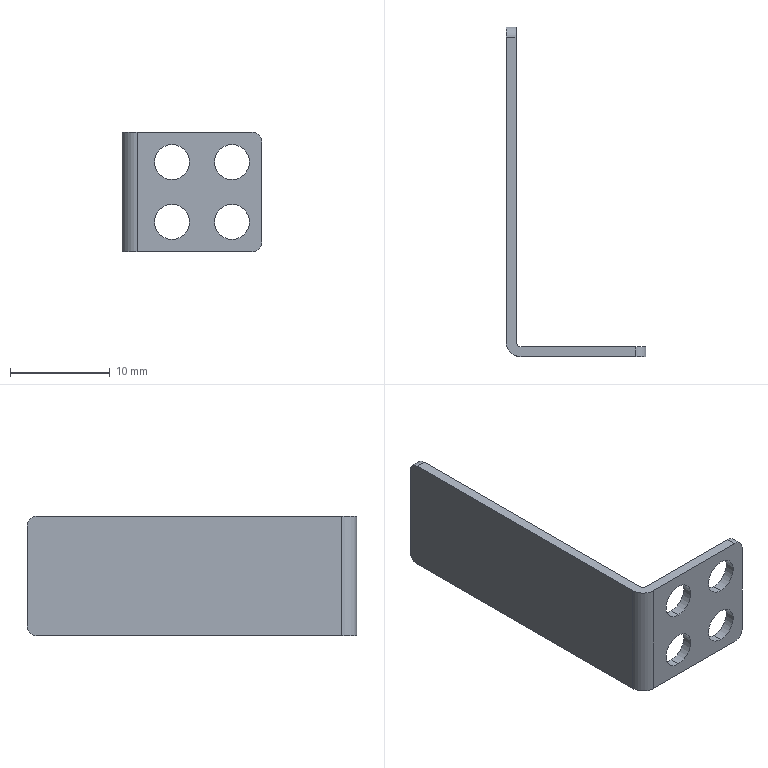Part | SolidWorks | features MoveFace 7, ICE 2, BaseBody 1, Fillet 1 | 1 solid | 22 faces | box 14 x 33 x 12 mm | volume 507.507 mm3 | cylinder 14 | plane 8 | commonest cylinder face diameters 3.5 x8 2 x4 1 x1 3 x1
STEP:
#1=CARTESIAN_POINT('',(4.,-12.5,-9.25));
#2=VERTEX_POINT('',#1);
#3=CARTESIAN_POINT('',(4.,-12.5,-12.75));
#4=VERTEX_POINT('',#3);
#5=CARTESIAN_POINT('',(4.,-12.5,-11.));
#6=DIRECTION('',(0.,-1.,0.));
#7=DIRECTION('',(0.,0.,-1.));
#8=AXIS2_PLACEMENT_3D('',#5,#6,#7);
#9=CIRCLE('',#8,1.75);
#10=EDGE_CURVE('',#2,#4,#9,.T.);
#11=ORIENTED_EDGE('',*,*,#10,.T.);
#12=CARTESIAN_POINT('',(4.,-11.5,-12.75));
#13=VERTEX_POINT('',#12);
#14=CARTESIAN_POINT('',(4.,-21.5,-12.75));
#15=DIRECTION('',(0.,1.,0.));
#16=VECTOR('',#15,1000.);
#17=LINE('',#14,#16);
#18=EDGE_CURVE('',#4,#13,#17,.T.);
#19=ORIENTED_EDGE('',*,*,#18,.T.);
#20=CARTESIAN_POINT('',(4.,-11.5,-9.25));
#21=VERTEX_POINT('',#20);
#22=CARTESIAN_POINT('',(4.,-11.5,-11.));
#23=DIRECTION('',(0.,1.,0.));
#24=DIRECTION('',(0.,0.,1.));
#25=AXIS2_PLACEMENT_3D('',#22,#23,#24);
#26=CIRCLE('',#25,1.75);
#27=EDGE_CURVE('',#13,#21,#26,.T.);
#28=ORIENTED_EDGE('',*,*,#27,.T.);
#29=CARTESIAN_POINT('',(4.,-21.5,-9.25));
#30=DIRECTION('',(0.,1.,0.));
#31=VECTOR('',#30,1000.);
#32=LINE('',#29,#31);
#33=EDGE_CURVE('',#2,#21,#32,.T.);
#34=ORIENTED_EDGE('',*,*,#33,.F.);
#35=EDGE_LOOP('',(#11,#19,#28,#34));
#36=FACE_OUTER_BOUND('',#35,.T.);
#37=CARTESIAN_POINT('',(4.,-21.5,-11.));
#38=DIRECTION('',(0.,1.,0.));
#39=DIRECTION('',(0.,0.,1.));
#40=AXIS2_PLACEMENT_3D('',#37,#38,#39);
#41=CYLINDRICAL_SURFACE('',#40,1.75);
#42=ADVANCED_FACE('',(#36),#41,.F.);
#43=CARTESIAN_POINT('',(-2.,-12.5,-12.75));
#44=VERTEX_POINT('',#43);
#45=CARTESIAN_POINT('',(-2.,-12.5,-9.25));
#46=VERTEX_POINT('',#45);
#47=CARTESIAN_POINT('',(-2.,-12.5,-11.));
#48=DIRECTION('',(0.,1.,0.));
#49=DIRECTION('',(0.,0.,1.));
#50=AXIS2_PLACEMENT_3D('',#47,#48,#49);
#51=CIRCLE('',#50,1.75);
#52=EDGE_CURVE('',#44,#46,#51,.T.);
#53=ORIENTED_EDGE('',*,*,#52,.F.);
#54=CARTESIAN_POINT('',(-2.,-11.5,-12.75));
#55=VERTEX_POINT('',#54);
#56=CARTESIAN_POINT('',(-2.,-11.5,-12.75));
#57=DIRECTION('',(0.,1.,0.));
#58=VECTOR('',#57,1000.);
#59=LINE('',#56,#58);
#60=EDGE_CURVE('',#44,#55,#59,.T.);
#61=ORIENTED_EDGE('',*,*,#60,.T.);
#62=CARTESIAN_POINT('',(-2.,-11.5,-9.25));
#63=VERTEX_POINT('',#62);
#64=CARTESIAN_POINT('',(-2.,-11.5,-11.));
#65=DIRECTION('',(0.,1.,0.));
#66=DIRECTION('',(0.,0.,1.));
#67=AXIS2_PLACEMENT_3D('',#64,#65,#66);
#68=CIRCLE('',#67,1.75);
#69=EDGE_CURVE('',#55,#63,#68,.T.);
#70=ORIENTED_EDGE('',*,*,#69,.T.);
#71=CARTESIAN_POINT('',(-2.,-11.5,-9.25));
#72=DIRECTION('',(0.,1.,0.));
#73=VECTOR('',#72,1000.);
#74=LINE('',#71,#73);
#75=EDGE_CURVE('',#46,#63,#74,.T.);
#76=ORIENTED_EDGE('',*,*,#75,.F.);
#77=EDGE_LOOP('',(#53,#61,#70,#76));
#78=FACE_OUTER_BOUND('',#77,.T.);
#79=CARTESIAN_POINT('',(-2.,-11.5,-11.));
#80=DIRECTION('',(0.,1.,0.));
#81=DIRECTION('',(0.,0.,1.));
#82=AXIS2_PLACEMENT_3D('',#79,#80,#81);
#83=CYLINDRICAL_SURFACE('',#82,1.75);
#84=ADVANCED_FACE('',(#78),#83,.F.);
#85=CARTESIAN_POINT('',(4.,-12.5,-6.75));
#86=VERTEX_POINT('',#85);
#87=CARTESIAN_POINT('',(4.,-12.5,-3.25));
#88=VERTEX_POINT('',#87);
#89=CARTESIAN_POINT('',(4.,-12.5,-5.));
#90=DIRECTION('',(0.,1.,0.));
#91=DIRECTION('',(0.,0.,1.));
#92=AXIS2_PLACEMENT_3D('',#89,#90,#91);
#93=CIRCLE('',#92,1.75);
#94=EDGE_CURVE('',#86,#88,#93,.T.);
#95=ORIENTED_EDGE('',*,*,#94,.F.);
#96=CARTESIAN_POINT('',(4.,-11.5,-6.75));
#97=VERTEX_POINT('',#96);
#98=CARTESIAN_POINT('',(4.,-11.5,-6.75));
#99=DIRECTION('',(0.,1.,0.));
#100=VECTOR('',#99,1000.);
#101=LINE('',#98,#100);
#102=EDGE_CURVE('',#86,#97,#101,.T.);
#103=ORIENTED_EDGE('',*,*,#102,.T.);
#104=CARTESIAN_POINT('',(4.,-11.5,-3.25));
#105=VERTEX_POINT('',#104);
#106=CARTESIAN_POINT('',(4.,-11.5,-5.));
#107=DIRECTION('',(0.,1.,0.));
#108=DIRECTION('',(0.,0.,1.));
#109=AXIS2_PLACEMENT_3D('',#106,#107,#108);
#110=CIRCLE('',#109,1.75);
#111=EDGE_CURVE('',#97,#105,#110,.T.);
#112=ORIENTED_EDGE('',*,*,#111,.T.);
#113=CARTESIAN_POINT('',(4.,-11.5,-3.25));
#114=DIRECTION('',(0.,1.,0.));
#115=VECTOR('',#114,1000.);
#116=LINE('',#113,#115);
#117=EDGE_CURVE('',#88,#105,#116,.T.);
#118=ORIENTED_EDGE('',*,*,#117,.F.);
#119=EDGE_LOOP('',(#95,#103,#112,#118));
#120=FACE_OUTER_BOUND('',#119,.T.);
#121=CARTESIAN_POINT('',(4.,-11.5,-5.));
#122=DIRECTION('',(0.,1.,0.));
#123=DIRECTION('',(0.,0.,1.));
#124=AXIS2_PLACEMENT_3D('',#121,#122,#123);
#125=CYLINDRICAL_SURFACE('',#124,1.75);
#126=ADVANCED_FACE('',(#120),#125,.F.);
#127=CARTESIAN_POINT('',(-2.,-12.5,-6.75));
#128=VERTEX_POINT('',#127);
#129=CARTESIAN_POINT('',(-2.,-12.5,-3.25));
#130=VERTEX_POINT('',#129);
#131=CARTESIAN_POINT('',(-2.,-12.5,-5.));
#132=DIRECTION('',(0.,1.,0.));
#133=DIRECTION('',(0.,0.,1.));
#134=AXIS2_PLACEMENT_3D('',#131,#132,#133);
#135=CIRCLE('',#134,1.75);
#136=EDGE_CURVE('',#128,#130,#135,.T.);
#137=ORIENTED_EDGE('',*,*,#136,.F.);
#138=CARTESIAN_POINT('',(-2.,-11.5,-6.75));
#139=VERTEX_POINT('',#138);
#140=CARTESIAN_POINT('',(-2.,-11.5,-6.75));
#141=DIRECTION('',(0.,1.,0.));
#142=VECTOR('',#141,1000.);
#143=LINE('',#140,#142);
#144=EDGE_CURVE('',#128,#139,#143,.T.);
#145=ORIENTED_EDGE('',*,*,#144,.T.);
#146=CARTESIAN_POINT('',(-2.,-11.5,-3.25));
#147=VERTEX_POINT('',#146);
#148=CARTESIAN_POINT('',(-2.,-11.5,-5.));
#149=DIRECTION('',(0.,1.,0.));
#150=DIRECTION('',(0.,0.,1.));
#151=AXIS2_PLACEMENT_3D('',#148,#149,#150);
#152=CIRCLE('',#151,1.75);
#153=EDGE_CURVE('',#139,#147,#152,.T.);
#154=ORIENTED_EDGE('',*,*,#153,.T.);
#155=CARTESIAN_POINT('',(-2.,-11.5,-3.25));
#156=DIRECTION('',(0.,1.,0.));
#157=VECTOR('',#156,1000.);
#158=LINE('',#155,#157);
#159=EDGE_CURVE('',#130,#147,#158,.T.);
#160=ORIENTED_EDGE('',*,*,#159,.F.);
#161=EDGE_LOOP('',(#137,#145,#154,#160));
#162=FACE_OUTER_BOUND('',#161,.T.);
#163=CARTESIAN_POINT('',(-2.,-11.5,-5.));
#164=DIRECTION('',(0.,1.,0.));
#165=DIRECTION('',(0.,0.,1.));
#166=AXIS2_PLACEMENT_3D('',#163,#164,#165);
#167=CYLINDRICAL_SURFACE('',#166,1.75);
#168=ADVANCED_FACE('',(#162),#167,.F.);
#169=CARTESIAN_POINT('',(-6.,20.5,-13.));
#170=VERTEX_POINT('',#169);
#171=CARTESIAN_POINT('',(-6.,19.5,-14.));
#172=VERTEX_POINT('',#171);
#173=CARTESIAN_POINT('',(-6.,19.5,-13.));
#174=DIRECTION('',(-1.,0.,0.));
#175=DIRECTION('',(0.,0.,-1.));
#176=AXIS2_PLACEMENT_3D('',#173,#174,#175);
#177=CIRCLE('',#176,1.);
#178=EDGE_CURVE('',#170,#172,#177,.T.);
#179=ORIENTED_EDGE('',*,*,#178,.F.);
#180=CARTESIAN_POINT('',(-6.,20.5,-3.));
#181=VERTEX_POINT('',#180);
#182=CARTESIAN_POINT('',(-6.,20.5,-15.));
#183=DIRECTION('',(0.,0.,-1.));
#184=VECTOR('',#183,1000.);
#185=LINE('',#182,#184);
#186=EDGE_CURVE('',#181,#170,#185,.T.);
#187=ORIENTED_EDGE('',*,*,#186,.F.);
#188=CARTESIAN_POINT('',(-6.,19.5,-2.));
#189=VERTEX_POINT('',#188);
#190=CARTESIAN_POINT('',(-6.,19.5,-3.));
#191=DIRECTION('',(-1.,0.,0.));
#192=DIRECTION('',(0.,0.,1.));
#193=AXIS2_PLACEMENT_3D('',#190,#191,#192);
#194=CIRCLE('',#193,1.);
#195=EDGE_CURVE('',#189,#181,#194,.T.);
#196=ORIENTED_EDGE('',*,*,#195,.F.);
#197=CARTESIAN_POINT('',(-6.,-11.,-2.));
#198=VERTEX_POINT('',#197);
#199=CARTESIAN_POINT('',(-6.,25.632,-2.));
#200=DIRECTION('',(0.,1.,0.));
#201=VECTOR('',#200,1000.);
#202=LINE('',#199,#201);
#203=EDGE_CURVE('',#198,#189,#202,.T.);
#204=ORIENTED_EDGE('',*,*,#203,.F.);
#205=CARTESIAN_POINT('',(-6.,-11.,-14.));
#206=VERTEX_POINT('',#205);
#207=CARTESIAN_POINT('',(-6.,-11.,-15.));
#208=DIRECTION('',(0.,0.,1.));
#209=VECTOR('',#208,1000.);
#210=LINE('',#207,#209);
#211=EDGE_CURVE('',#206,#198,#210,.T.);
#212=ORIENTED_EDGE('',*,*,#211,.F.);
#213=CARTESIAN_POINT('',(-6.,25.632,-14.));
#214=DIRECTION('',(0.,-1.,0.));
#215=VECTOR('',#214,1000.);
#216=LINE('',#213,#215);
#217=EDGE_CURVE('',#172,#206,#216,.T.);
#218=ORIENTED_EDGE('',*,*,#217,.F.);
#219=EDGE_LOOP('',(#179,#187,#196,#204,#212,#218));
#220=FACE_OUTER_BOUND('',#219,.T.);
#221=CARTESIAN_POINT('',(-6.,25.632,-15.));
#222=DIRECTION('',(-1.,0.,0.));
#223=DIRECTION('',(0.,-1.,0.));
#224=AXIS2_PLACEMENT_3D('',#221,#222,#223);
#225=PLANE('',#224);
#226=ADVANCED_FACE('',(#220),#225,.F.);
#227=CARTESIAN_POINT('',(-5.5,-11.5,-14.));
#228=VERTEX_POINT('',#227);
#229=CARTESIAN_POINT('',(6.,-11.5,-14.));
#230=VERTEX_POINT('',#229);
#231=CARTESIAN_POINT('',(28.84,-11.5,-14.));
#232=DIRECTION('',(1.,0.,0.));
#233=VECTOR('',#232,1000.);
#234=LINE('',#231,#233);
#235=EDGE_CURVE('',#228,#230,#234,.T.);
#236=ORIENTED_EDGE('',*,*,#235,.T.);
#237=CARTESIAN_POINT('',(6.,-12.5,-14.));
#238=VERTEX_POINT('',#237);
#239=CARTESIAN_POINT('',(6.,-12.5,-14.));
#240=DIRECTION('',(0.,-1.,0.));
#241=VECTOR('',#240,1000.);
#242=LINE('',#239,#241);
#243=EDGE_CURVE('',#230,#238,#242,.T.);
#244=ORIENTED_EDGE('',*,*,#243,.T.);
#245=CARTESIAN_POINT('',(-5.5,-12.5,-14.));
#246=VERTEX_POINT('',#245);
#247=CARTESIAN_POINT('',(-7.,-12.5,-14.));
#248=DIRECTION('',(1.,0.,0.));
#249=VECTOR('',#248,1000.);
#250=LINE('',#247,#249);
#251=EDGE_CURVE('',#246,#238,#250,.T.);
#252=ORIENTED_EDGE('',*,*,#251,.F.);
#253=CARTESIAN_POINT('',(-7.,-11.,-14.));
#254=VERTEX_POINT('',#253);
#255=CARTESIAN_POINT('',(-5.5,-11.,-14.));
#256=DIRECTION('',(0.,0.,1.));
#257=DIRECTION('',(1.,0.,0.));
#258=AXIS2_PLACEMENT_3D('',#255,#256,#257);
#259=CIRCLE('',#258,1.5);
#260=EDGE_CURVE('',#254,#246,#259,.T.);
#261=ORIENTED_EDGE('',*,*,#260,.F.);
#262=CARTESIAN_POINT('',(-7.,19.5,-14.));
#263=VERTEX_POINT('',#262);
#264=CARTESIAN_POINT('',(-7.,12.5,-14.));
#265=DIRECTION('',(0.,-1.,0.));
#266=VECTOR('',#265,1000.);
#267=LINE('',#264,#266);
#268=EDGE_CURVE('',#263,#254,#267,.T.);
#269=ORIENTED_EDGE('',*,*,#268,.F.);
#270=CARTESIAN_POINT('',(-5.,19.5,-14.));
#271=DIRECTION('',(-1.,0.,0.));
#272=VECTOR('',#271,1000.);
#273=LINE('',#270,#272);
#274=EDGE_CURVE('',#172,#263,#273,.T.);
#275=ORIENTED_EDGE('',*,*,#274,.F.);
#276=ORIENTED_EDGE('',*,*,#217,.T.);
#277=CARTESIAN_POINT('',(-5.5,-11.,-14.));
#278=DIRECTION('',(0.,0.,-1.));
#279=DIRECTION('',(-1.,0.,0.));
#280=AXIS2_PLACEMENT_3D('',#277,#278,#279);
#281=CIRCLE('',#280,0.5);
#282=EDGE_CURVE('',#228,#206,#281,.T.);
#283=ORIENTED_EDGE('',*,*,#282,.F.);
#284=EDGE_LOOP('',(#236,#244,#252,#261,#269,#275,#276,#283));
#285=FACE_OUTER_BOUND('',#284,.T.);
#286=CARTESIAN_POINT('',(-5.,12.5,-14.));
#287=DIRECTION('',(0.,0.,1.));
#288=DIRECTION('',(1.,0.,0.));
#289=AXIS2_PLACEMENT_3D('',#286,#287,#288);
#290=PLANE('',#289);
#291=ADVANCED_FACE('',(#285),#290,.F.);
#292=CARTESIAN_POINT('',(-7.,20.5,-13.));
#293=VERTEX_POINT('',#292);
#294=CARTESIAN_POINT('',(-7.,19.5,-13.));
#295=DIRECTION('',(1.,0.,0.));
#296=DIRECTION('',(0.,0.,-1.));
#297=AXIS2_PLACEMENT_3D('',#294,#295,#296);
#298=CIRCLE('',#297,1.);
#299=EDGE_CURVE('',#263,#293,#298,.T.);
#300=ORIENTED_EDGE('',*,*,#299,.T.);
#301=CARTESIAN_POINT('',(-7.,20.5,-13.));
#302=DIRECTION('',(1.,0.,0.));
#303=VECTOR('',#302,1000.);
#304=LINE('',#301,#303);
#305=EDGE_CURVE('',#293,#170,#304,.T.);
#306=ORIENTED_EDGE('',*,*,#305,.T.);
#307=ORIENTED_EDGE('',*,*,#178,.T.);
#308=ORIENTED_EDGE('',*,*,#274,.T.);
#309=EDGE_LOOP('',(#300,#306,#307,#308));
#310=FACE_OUTER_BOUND('',#309,.T.);
#311=CARTESIAN_POINT('',(-7.,19.5,-13.));
#312=DIRECTION('',(1.,0.,0.));
#313=DIRECTION('',(0.,0.,-1.));
#314=AXIS2_PLACEMENT_3D('',#311,#312,#313);
#315=CYLINDRICAL_SURFACE('',#314,1.);
#316=ADVANCED_FACE('',(#310),#315,.T.);
#317=CARTESIAN_POINT('',(-7.,20.5,-3.));
#318=VERTEX_POINT('',#317);
#319=CARTESIAN_POINT('',(-7.,20.5,-15.));
#320=DIRECTION('',(0.,0.,1.));
#321=VECTOR('',#320,1000.);
#322=LINE('',#319,#321);
#323=EDGE_CURVE('',#293,#318,#322,.T.);
#324=ORIENTED_EDGE('',*,*,#323,.T.);
#325=CARTESIAN_POINT('',(-7.,20.5,-3.));
#326=DIRECTION('',(1.,0.,0.));
#327=VECTOR('',#326,1000.);
#328=LINE('',#325,#327);
#329=EDGE_CURVE('',#318,#181,#328,.T.);
#330=ORIENTED_EDGE('',*,*,#329,.T.);
#331=ORIENTED_EDGE('',*,*,#186,.T.);
#332=ORIENTED_EDGE('',*,*,#305,.F.);
#333=EDGE_LOOP('',(#324,#330,#331,#332));
#334=FACE_OUTER_BOUND('',#333,.T.);
#335=CARTESIAN_POINT('',(-7.,20.5,-15.));
#336=DIRECTION('',(0.,1.,0.));
#337=DIRECTION('',(0.,0.,1.));
#338=AXIS2_PLACEMENT_3D('',#335,#336,#337);
#339=PLANE('',#338);
#340=ADVANCED_FACE('',(#334),#339,.T.);
#341=CARTESIAN_POINT('',(-7.,19.5,-2.));
#342=VERTEX_POINT('',#341);
#343=CARTESIAN_POINT('',(-7.,19.5,-3.));
#344=DIRECTION('',(1.,0.,0.));
#345=DIRECTION('',(0.,0.,1.));
#346=AXIS2_PLACEMENT_3D('',#343,#344,#345);
#347=CIRCLE('',#346,1.);
#348=EDGE_CURVE('',#318,#342,#347,.T.);
#349=ORIENTED_EDGE('',*,*,#348,.T.);
#350=CARTESIAN_POINT('',(0.,19.5,-2.));
#351=DIRECTION('',(1.,0.,0.));
#352=VECTOR('',#351,1000.);
#353=LINE('',#350,#352);
#354=EDGE_CURVE('',#342,#189,#353,.T.);
#355=ORIENTED_EDGE('',*,*,#354,.T.);
#356=ORIENTED_EDGE('',*,*,#195,.T.);
#357=ORIENTED_EDGE('',*,*,#329,.F.);
#358=EDGE_LOOP('',(#349,#355,#356,#357));
#359=FACE_OUTER_BOUND('',#358,.T.);
#360=CARTESIAN_POINT('',(0.,19.5,-3.));
#361=DIRECTION('',(-1.,0.,0.));
#362=DIRECTION('',(0.,0.,1.));
#363=AXIS2_PLACEMENT_3D('',#360,#361,#362);
#364=CYLINDRICAL_SURFACE('',#363,1.);
#365=ADVANCED_FACE('',(#359),#364,.T.);
#366=CARTESIAN_POINT('',(6.,-11.5,-2.));
#367=VERTEX_POINT('',#366);
#368=CARTESIAN_POINT('',(-5.5,-11.5,-2.));
#369=VERTEX_POINT('',#368);
#370=CARTESIAN_POINT('',(0.,-11.5,-2.));
#371=DIRECTION('',(-1.,0.,0.));
#372=VECTOR('',#371,1000.);
#373=LINE('',#370,#372);
#374=EDGE_CURVE('',#367,#369,#373,.T.);
#375=ORIENTED_EDGE('',*,*,#374,.T.);
#376=CARTESIAN_POINT('',(-5.5,-11.,-2.));
#377=DIRECTION('',(0.,0.,-1.));
#378=DIRECTION('',(-1.,0.,0.));
#379=AXIS2_PLACEMENT_3D('',#376,#377,#378);
#380=CIRCLE('',#379,0.5);
#381=EDGE_CURVE('',#369,#198,#380,.T.);
#382=ORIENTED_EDGE('',*,*,#381,.T.);
#383=ORIENTED_EDGE('',*,*,#203,.T.);
#384=ORIENTED_EDGE('',*,*,#354,.F.);
#385=CARTESIAN_POINT('',(-7.,-11.,-2.));
#386=VERTEX_POINT('',#385);
#387=CARTESIAN_POINT('',(-7.,0.,-2.));
#388=DIRECTION('',(0.,-1.,0.));
#389=VECTOR('',#388,1000.);
#390=LINE('',#387,#389);
#391=EDGE_CURVE('',#342,#386,#390,.T.);
#392=ORIENTED_EDGE('',*,*,#391,.T.);
#393=CARTESIAN_POINT('',(-5.5,-12.5,-2.));
#394=VERTEX_POINT('',#393);
#395=CARTESIAN_POINT('',(-5.5,-11.,-2.));
#396=DIRECTION('',(0.,0.,1.));
#397=DIRECTION('',(1.,0.,0.));
#398=AXIS2_PLACEMENT_3D('',#395,#396,#397);
#399=CIRCLE('',#398,1.5);
#400=EDGE_CURVE('',#386,#394,#399,.T.);
#401=ORIENTED_EDGE('',*,*,#400,.T.);
#402=CARTESIAN_POINT('',(6.,-12.5,-2.));
#403=VERTEX_POINT('',#402);
#404=CARTESIAN_POINT('',(0.,-12.5,-2.));
#405=DIRECTION('',(1.,0.,0.));
#406=VECTOR('',#405,1000.);
#407=LINE('',#404,#406);
#408=EDGE_CURVE('',#394,#403,#407,.T.);
#409=ORIENTED_EDGE('',*,*,#408,.T.);
#410=CARTESIAN_POINT('',(6.,0.,-2.));
#411=DIRECTION('',(0.,1.,0.));
#412=VECTOR('',#411,1000.);
#413=LINE('',#410,#412);
#414=EDGE_CURVE('',#403,#367,#413,.T.);
#415=ORIENTED_EDGE('',*,*,#414,.T.);
#416=EDGE_LOOP('',(#375,#382,#383,#384,#392,#401,#409,#415));
#417=FACE_OUTER_BOUND('',#416,.T.);
#418=CARTESIAN_POINT('',(0.,0.,-2.));
#419=DIRECTION('',(0.,0.,1.));
#420=DIRECTION('',(1.,0.,0.));
#421=AXIS2_PLACEMENT_3D('',#418,#419,#420);
#422=PLANE('',#421);
#423=ADVANCED_FACE('',(#417),#422,.T.);
#424=ORIENTED_EDGE('',*,*,#282,.T.);
#425=ORIENTED_EDGE('',*,*,#211,.T.);
#426=ORIENTED_EDGE('',*,*,#381,.F.);
#427=CARTESIAN_POINT('',(-5.5,-11.5,-15.));
#428=DIRECTION('',(0.,0.,1.));
#429=VECTOR('',#428,1000.);
#430=LINE('',#427,#429);
#431=EDGE_CURVE('',#228,#369,#430,.T.);
#432=ORIENTED_EDGE('',*,*,#431,.F.);
#433=EDGE_LOOP('',(#424,#425,#426,#432));
#434=FACE_OUTER_BOUND('',#433,.T.);
#435=CARTESIAN_POINT('',(-5.5,-11.,-15.));
#436=DIRECTION('',(0.,0.,-1.));
#437=DIRECTION('',(-1.,0.,0.));
#438=AXIS2_PLACEMENT_3D('',#435,#436,#437);
#439=CYLINDRICAL_SURFACE('',#438,0.5);
#440=ADVANCED_FACE('',(#434),#439,.F.);
#441=ORIENTED_EDGE('',*,*,#391,.F.);
#442=ORIENTED_EDGE('',*,*,#348,.F.);
#443=ORIENTED_EDGE('',*,*,#323,.F.);
#444=ORIENTED_EDGE('',*,*,#299,.F.);
#445=ORIENTED_EDGE('',*,*,#268,.T.);
#446=CARTESIAN_POINT('',(-7.,-11.,-15.));
#447=DIRECTION('',(0.,0.,1.));
#448=VECTOR('',#447,1000.);
#449=LINE('',#446,#448);
#450=EDGE_CURVE('',#254,#386,#449,.T.);
#451=ORIENTED_EDGE('',*,*,#450,.T.);
#452=EDGE_LOOP('',(#441,#442,#443,#444,#445,#451));
#453=FACE_OUTER_BOUND('',#452,.T.);
#454=CARTESIAN_POINT('',(-7.,12.5,-15.));
#455=DIRECTION('',(-1.,0.,0.));
#456=DIRECTION('',(0.,-1.,0.));
#457=AXIS2_PLACEMENT_3D('',#454,#455,#456);
#458=PLANE('',#457);
#459=ADVANCED_FACE('',(#453),#458,.T.);
#460=ORIENTED_EDGE('',*,*,#400,.F.);
#461=ORIENTED_EDGE('',*,*,#450,.F.);
#462=ORIENTED_EDGE('',*,*,#260,.T.);
#463=CARTESIAN_POINT('',(-5.5,-12.5,-15.));
#464=DIRECTION('',(0.,0.,1.));
#465=VECTOR('',#464,1000.);
#466=LINE('',#463,#465);
#467=EDGE_CURVE('',#246,#394,#466,.T.);
#468=ORIENTED_EDGE('',*,*,#467,.T.);
#469=EDGE_LOOP('',(#460,#461,#462,#468));
#470=FACE_OUTER_BOUND('',#469,.T.);
#471=CARTESIAN_POINT('',(-5.5,-11.,-15.));
#472=DIRECTION('',(0.,0.,1.));
#473=DIRECTION('',(1.,0.,0.));
#474=AXIS2_PLACEMENT_3D('',#471,#472,#473);
#475=CYLINDRICAL_SURFACE('',#474,1.5);
#476=ADVANCED_FACE('',(#470),#475,.T.);
#477=CARTESIAN_POINT('',(4.,-11.5,-11.));
#478=DIRECTION('',(0.,1.,0.));
#479=DIRECTION('',(0.,0.,1.));
#480=AXIS2_PLACEMENT_3D('',#477,#478,#479);
#481=CIRCLE('',#480,1.75);
#482=EDGE_CURVE('',#21,#13,#481,.T.);
#483=ORIENTED_EDGE('',*,*,#482,.F.);
#484=ORIENTED_EDGE('',*,*,#27,.F.);
#485=EDGE_LOOP('',(#483,#484));
#486=FACE_BOUND('',#485,.T.);
#487=CARTESIAN_POINT('',(7.,-11.5,-13.));
#488=VERTEX_POINT('',#487);
#489=CARTESIAN_POINT('',(7.,-11.5,-3.));
#490=VERTEX_POINT('',#489);
#491=CARTESIAN_POINT('',(7.,-11.5,-15.));
#492=DIRECTION('',(0.,0.,1.));
#493=VECTOR('',#492,1000.);
#494=LINE('',#491,#493);
#495=EDGE_CURVE('',#488,#490,#494,.T.);
#496=ORIENTED_EDGE('',*,*,#495,.F.);
#497=CARTESIAN_POINT('',(6.,-11.5,-13.));
#498=DIRECTION('',(0.,1.,0.));
#499=DIRECTION('',(0.,0.,-1.));
#500=AXIS2_PLACEMENT_3D('',#497,#498,#499);
#501=CIRCLE('',#500,1.);
#502=EDGE_CURVE('',#488,#230,#501,.T.);
#503=ORIENTED_EDGE('',*,*,#502,.T.);
#504=ORIENTED_EDGE('',*,*,#235,.F.);
#505=ORIENTED_EDGE('',*,*,#431,.T.);
#506=ORIENTED_EDGE('',*,*,#374,.F.);
#507=CARTESIAN_POINT('',(6.,-11.5,-3.));
#508=DIRECTION('',(0.,-1.,0.));
#509=DIRECTION('',(-1.,0.,0.));
#510=AXIS2_PLACEMENT_3D('',#507,#508,#509);
#511=CIRCLE('',#510,1.);
#512=EDGE_CURVE('',#490,#367,#511,.T.);
#513=ORIENTED_EDGE('',*,*,#512,.F.);
#514=EDGE_LOOP('',(#496,#503,#504,#505,#506,#513));
#515=FACE_OUTER_BOUND('',#514,.T.);
#516=CARTESIAN_POINT('',(-2.,-11.5,-11.));
#517=DIRECTION('',(0.,1.,0.));
#518=DIRECTION('',(0.,0.,1.));
#519=AXIS2_PLACEMENT_3D('',#516,#517,#518);
#520=CIRCLE('',#519,1.75);
#521=EDGE_CURVE('',#63,#55,#520,.T.);
#522=ORIENTED_EDGE('',*,*,#521,.F.);
#523=ORIENTED_EDGE('',*,*,#69,.F.);
#524=EDGE_LOOP('',(#522,#523));
#525=FACE_BOUND('',#524,.T.);
#526=CARTESIAN_POINT('',(4.,-11.5,-5.));
#527=DIRECTION('',(0.,1.,0.));
#528=DIRECTION('',(0.,0.,1.));
#529=AXIS2_PLACEMENT_3D('',#526,#527,#528);
#530=CIRCLE('',#529,1.75);
#531=EDGE_CURVE('',#105,#97,#530,.T.);
#532=ORIENTED_EDGE('',*,*,#531,.F.);
#533=ORIENTED_EDGE('',*,*,#111,.F.);
#534=EDGE_LOOP('',(#532,#533));
#535=FACE_BOUND('',#534,.T.);
#536=CARTESIAN_POINT('',(-2.,-11.5,-5.));
#537=DIRECTION('',(0.,1.,0.));
#538=DIRECTION('',(0.,0.,1.));
#539=AXIS2_PLACEMENT_3D('',#536,#537,#538);
#540=CIRCLE('',#539,1.75);
#541=EDGE_CURVE('',#147,#139,#540,.T.);
#542=ORIENTED_EDGE('',*,*,#541,.F.);
#543=ORIENTED_EDGE('',*,*,#153,.F.);
#544=EDGE_LOOP('',(#542,#543));
#545=FACE_BOUND('',#544,.T.);
#546=CARTESIAN_POINT('',(28.84,-11.5,-15.));
#547=DIRECTION('',(0.,-1.,0.));
#548=DIRECTION('',(0.,0.,-1.));
#549=AXIS2_PLACEMENT_3D('',#546,#547,#548);
#550=PLANE('',#549);
#551=ADVANCED_FACE('',(#486,#515,#525,#535,#545),#550,.F.);
#552=ORIENTED_EDGE('',*,*,#512,.T.);
#553=ORIENTED_EDGE('',*,*,#414,.F.);
#554=CARTESIAN_POINT('',(7.,-12.5,-3.));
#555=VERTEX_POINT('',#554);
#556=CARTESIAN_POINT('',(6.,-12.5,-3.));
#557=DIRECTION('',(0.,1.,0.));
#558=DIRECTION('',(-1.,0.,0.));
#559=AXIS2_PLACEMENT_3D('',#556,#557,#558);
#560=CIRCLE('',#559,1.);
#561=EDGE_CURVE('',#403,#555,#560,.T.);
#562=ORIENTED_EDGE('',*,*,#561,.T.);
#563=CARTESIAN_POINT('',(7.,0.,-3.));
#564=DIRECTION('',(0.,1.,0.));
#565=VECTOR('',#564,1000.);
#566=LINE('',#563,#565);
#567=EDGE_CURVE('',#555,#490,#566,.T.);
#568=ORIENTED_EDGE('',*,*,#567,.T.);
#569=EDGE_LOOP('',(#552,#553,#562,#568));
#570=FACE_OUTER_BOUND('',#569,.T.);
#571=CARTESIAN_POINT('',(6.,0.,-3.));
#572=DIRECTION('',(0.,1.,0.));
#573=DIRECTION('',(-1.,0.,0.));
#574=AXIS2_PLACEMENT_3D('',#571,#572,#573);
#575=CYLINDRICAL_SURFACE('',#574,1.);
#576=ADVANCED_FACE('',(#570),#575,.T.);
#577=ORIENTED_EDGE('',*,*,#251,.T.);
#578=CARTESIAN_POINT('',(7.,-12.5,-13.));
#579=VERTEX_POINT('',#578);
#580=CARTESIAN_POINT('',(6.,-12.5,-13.));
#581=DIRECTION('',(0.,-1.,0.));
#582=DIRECTION('',(0.,0.,-1.));
#583=AXIS2_PLACEMENT_3D('',#580,#581,#582);
#584=CIRCLE('',#583,1.);
#585=EDGE_CURVE('',#238,#579,#584,.T.);
#586=ORIENTED_EDGE('',*,*,#585,.T.);
#587=CARTESIAN_POINT('',(7.,-12.5,-15.));
#588=DIRECTION('',(0.,0.,1.));
#589=VECTOR('',#588,1000.);
#590=LINE('',#587,#589);
#591=EDGE_CURVE('',#579,#555,#590,.T.);
#592=ORIENTED_EDGE('',*,*,#591,.T.);
#593=ORIENTED_EDGE('',*,*,#561,.F.);
#594=ORIENTED_EDGE('',*,*,#408,.F.);
#595=ORIENTED_EDGE('',*,*,#467,.F.);
#596=EDGE_LOOP('',(#577,#586,#592,#593,#594,#595));
#597=FACE_OUTER_BOUND('',#596,.T.);
#598=ORIENTED_EDGE('',*,*,#10,.F.);
#599=CARTESIAN_POINT('',(4.,-12.5,-11.));
#600=DIRECTION('',(0.,-1.,0.));
#601=DIRECTION('',(0.,0.,-1.));
#602=AXIS2_PLACEMENT_3D('',#599,#600,#601);
#603=CIRCLE('',#602,1.75);
#604=EDGE_CURVE('',#4,#2,#603,.T.);
#605=ORIENTED_EDGE('',*,*,#604,.F.);
#606=EDGE_LOOP('',(#598,#605));
#607=FACE_BOUND('',#606,.T.);
#608=CARTESIAN_POINT('',(-2.,-12.5,-11.));
#609=DIRECTION('',(0.,1.,0.));
#610=DIRECTION('',(0.,0.,1.));
#611=AXIS2_PLACEMENT_3D('',#608,#609,#610);
#612=CIRCLE('',#611,1.75);
#613=EDGE_CURVE('',#46,#44,#612,.T.);
#614=ORIENTED_EDGE('',*,*,#613,.T.);
#615=ORIENTED_EDGE('',*,*,#52,.T.);
#616=EDGE_LOOP('',(#614,#615));
#617=FACE_BOUND('',#616,.T.);
#618=CARTESIAN_POINT('',(4.,-12.5,-5.));
#619=DIRECTION('',(0.,1.,0.));
#620=DIRECTION('',(0.,0.,1.));
#621=AXIS2_PLACEMENT_3D('',#618,#619,#620);
#622=CIRCLE('',#621,1.75);
#623=EDGE_CURVE('',#88,#86,#622,.T.);
#624=ORIENTED_EDGE('',*,*,#623,.T.);
#625=ORIENTED_EDGE('',*,*,#94,.T.);
#626=EDGE_LOOP('',(#624,#625));
#627=FACE_BOUND('',#626,.T.);
#628=CARTESIAN_POINT('',(-2.,-12.5,-5.));
#629=DIRECTION('',(0.,1.,0.));
#630=DIRECTION('',(0.,0.,1.));
#631=AXIS2_PLACEMENT_3D('',#628,#629,#630);
#632=CIRCLE('',#631,1.75);
#633=EDGE_CURVE('',#130,#128,#632,.T.);
#634=ORIENTED_EDGE('',*,*,#633,.T.);
#635=ORIENTED_EDGE('',*,*,#136,.T.);
#636=EDGE_LOOP('',(#634,#635));
#637=FACE_BOUND('',#636,.T.);
#638=CARTESIAN_POINT('',(-7.,-12.5,-15.));
#639=DIRECTION('',(0.,-1.,0.));
#640=DIRECTION('',(0.,0.,-1.));
#641=AXIS2_PLACEMENT_3D('',#638,#639,#640);
#642=PLANE('',#641);
#643=ADVANCED_FACE('',(#597,#607,#617,#627,#637),#642,.T.);
#644=ORIENTED_EDGE('',*,*,#591,.F.);
#645=CARTESIAN_POINT('',(7.,-11.5,-13.));
#646=DIRECTION('',(0.,1.,0.));
#647=VECTOR('',#646,1000.);
#648=LINE('',#645,#647);
#649=EDGE_CURVE('',#579,#488,#648,.T.);
#650=ORIENTED_EDGE('',*,*,#649,.T.);
#651=ORIENTED_EDGE('',*,*,#495,.T.);
#652=ORIENTED_EDGE('',*,*,#567,.F.);
#653=EDGE_LOOP('',(#644,#650,#651,#652));
#654=FACE_OUTER_BOUND('',#653,.T.);
#655=CARTESIAN_POINT('',(7.,12.5,-15.));
#656=DIRECTION('',(1.,0.,0.));
#657=DIRECTION('',(0.,1.,0.));
#658=AXIS2_PLACEMENT_3D('',#655,#656,#657);
#659=PLANE('',#658);
#660=ADVANCED_FACE('',(#654),#659,.T.);
#661=ORIENTED_EDGE('',*,*,#60,.F.);
#662=ORIENTED_EDGE('',*,*,#613,.F.);
#663=ORIENTED_EDGE('',*,*,#75,.T.);
#664=ORIENTED_EDGE('',*,*,#521,.T.);
#665=EDGE_LOOP('',(#661,#662,#663,#664));
#666=FACE_OUTER_BOUND('',#665,.T.);
#667=CARTESIAN_POINT('',(-2.,-11.5,-11.));
#668=DIRECTION('',(0.,1.,0.));
#669=DIRECTION('',(0.,0.,1.));
#670=AXIS2_PLACEMENT_3D('',#667,#668,#669);
#671=CYLINDRICAL_SURFACE('',#670,1.75);
#672=ADVANCED_FACE('',(#666),#671,.F.);
#673=ORIENTED_EDGE('',*,*,#102,.F.);
#674=ORIENTED_EDGE('',*,*,#623,.F.);
#675=ORIENTED_EDGE('',*,*,#117,.T.);
#676=ORIENTED_EDGE('',*,*,#531,.T.);
#677=EDGE_LOOP('',(#673,#674,#675,#676));
#678=FACE_OUTER_BOUND('',#677,.T.);
#679=CARTESIAN_POINT('',(4.,-11.5,-5.));
#680=DIRECTION('',(0.,1.,0.));
#681=DIRECTION('',(0.,0.,1.));
#682=AXIS2_PLACEMENT_3D('',#679,#680,#681);
#683=CYLINDRICAL_SURFACE('',#682,1.75);
#684=ADVANCED_FACE('',(#678),#683,.F.);
#685=ORIENTED_EDGE('',*,*,#144,.F.);
#686=ORIENTED_EDGE('',*,*,#633,.F.);
#687=ORIENTED_EDGE('',*,*,#159,.T.);
#688=ORIENTED_EDGE('',*,*,#541,.T.);
#689=EDGE_LOOP('',(#685,#686,#687,#688));
#690=FACE_OUTER_BOUND('',#689,.T.);
#691=CARTESIAN_POINT('',(-2.,-11.5,-5.));
#692=DIRECTION('',(0.,1.,0.));
#693=DIRECTION('',(0.,0.,1.));
#694=AXIS2_PLACEMENT_3D('',#691,#692,#693);
#695=CYLINDRICAL_SURFACE('',#694,1.75);
#696=ADVANCED_FACE('',(#690),#695,.F.);
#697=ORIENTED_EDGE('',*,*,#18,.F.);
#698=ORIENTED_EDGE('',*,*,#604,.T.);
#699=ORIENTED_EDGE('',*,*,#33,.T.);
#700=ORIENTED_EDGE('',*,*,#482,.T.);
#701=EDGE_LOOP('',(#697,#698,#699,#700));
#702=FACE_OUTER_BOUND('',#701,.T.);
#703=CARTESIAN_POINT('',(4.,-21.5,-11.));
#704=DIRECTION('',(0.,1.,0.));
#705=DIRECTION('',(0.,0.,1.));
#706=AXIS2_PLACEMENT_3D('',#703,#704,#705);
#707=CYLINDRICAL_SURFACE('',#706,1.75);
#708=ADVANCED_FACE('',(#702),#707,.F.);
#709=ORIENTED_EDGE('',*,*,#502,.F.);
#710=ORIENTED_EDGE('',*,*,#649,.F.);
#711=ORIENTED_EDGE('',*,*,#585,.F.);
#712=ORIENTED_EDGE('',*,*,#243,.F.);
#713=EDGE_LOOP('',(#709,#710,#711,#712));
#714=FACE_OUTER_BOUND('',#713,.T.);
#715=CARTESIAN_POINT('',(6.,12.5,-13.));
#716=DIRECTION('',(0.,1.,0.));
#717=DIRECTION('',(-1.,0.,0.));
#718=AXIS2_PLACEMENT_3D('',#715,#716,#717);
#719=CYLINDRICAL_SURFACE('',#718,1.);
#720=ADVANCED_FACE('',(#714),#719,.T.);
#721=CLOSED_SHELL('',(#42,#84,#126,#168,#226,#291,#316,#340,#365,#423,#440,#459,#476,#551,#576,#643,#660,#672,#684,#696,#708,#720));
#722=MANIFOLD_SOLID_BREP('',#721);
#723=CARTESIAN_POINT('',(0.,0.,0.));
#724=DIRECTION('',(0.,0.,1.));
#725=DIRECTION('',(1.,0.,0.));
#726=AXIS2_PLACEMENT_3D('',#723,#724,#725);
#727=(LENGTH_UNIT()NAMED_UNIT(*)SI_UNIT(.MILLI.,.METRE.));
#728=UNCERTAINTY_MEASURE_WITH_UNIT(LENGTH_MEASURE(0.00001),#727,'','');
#729=(NAMED_UNIT(*)PLANE_ANGLE_UNIT()SI_UNIT($,.RADIAN.));
#730=(NAMED_UNIT(*)SI_UNIT($,.STERADIAN.)SOLID_ANGLE_UNIT());
#731=(GEOMETRIC_REPRESENTATION_CONTEXT(3)GLOBAL_UNCERTAINTY_ASSIGNED_CONTEXT((#728))GLOBAL_UNIT_ASSIGNED_CONTEXT((#727,#729,#730))REPRESENTATION_CONTEXT('',''));
#732=ADVANCED_BREP_SHAPE_REPRESENTATION('',(#722,#726),#731);